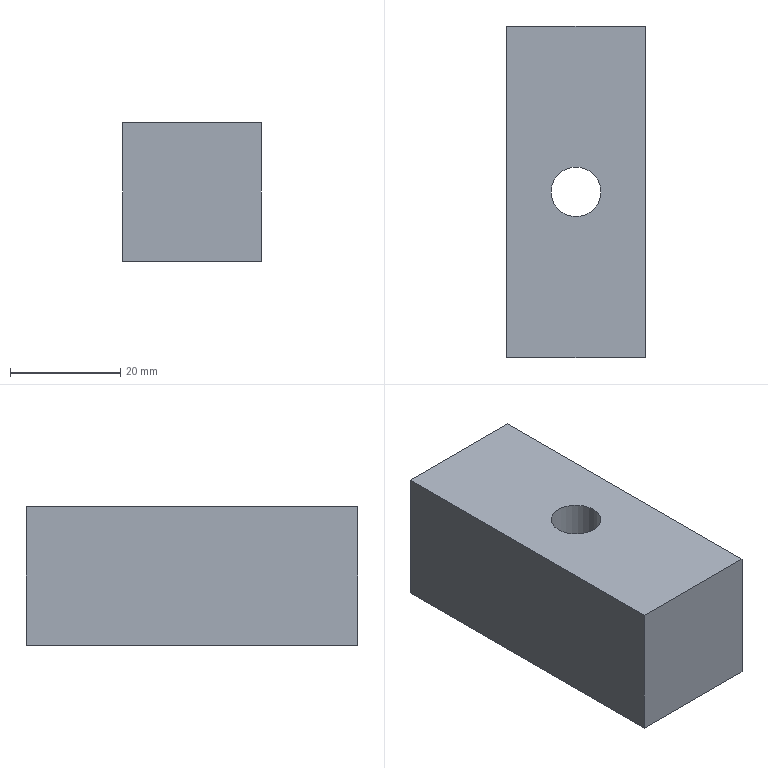Part | NX | features solid 2 | 1 solid | 9 faces | box 25 x 60 x 25 mm | volume 34555 mm3 | plane 7 | cylinder 2 | commonest cylinder face diameters 9 x1 14 x1
STEP:
#1=CARTESIAN_POINT('',(347.,484.5,118.));
#2=VERTEX_POINT('',#1);
#3=CARTESIAN_POINT('',(340.,484.5,118.));
#4=DIRECTION('',(0.,0.,1.));
#5=DIRECTION('',(1.,0.,0.));
#6=AXIS2_PLACEMENT_3D('',#3,#4,#5);
#7=CIRCLE('',#6,7.);
#8=EDGE_CURVE('',#2,#2,#7,.F.);
#9=ORIENTED_EDGE('',*,*,#8,.F.);
#10=EDGE_LOOP('',(#9));
#11=FACE_BOUND('',#10,.T.);
#12=CARTESIAN_POINT('',(327.5,514.5,118.));
#13=VERTEX_POINT('',#12);
#14=CARTESIAN_POINT('',(352.5,514.5,118.));
#15=VERTEX_POINT('',#14);
#16=CARTESIAN_POINT('',(330.,514.5,118.));
#17=DIRECTION('',(-1.,0.,0.));
#18=VECTOR('',#17,1000.);
#19=LINE('',#16,#18);
#20=EDGE_CURVE('',#13,#15,#19,.F.);
#21=ORIENTED_EDGE('',*,*,#20,.T.);
#22=CARTESIAN_POINT('',(352.5,454.5,118.));
#23=VERTEX_POINT('',#22);
#24=CARTESIAN_POINT('',(352.5,510.445,118.));
#25=DIRECTION('',(0.,-1.,0.));
#26=VECTOR('',#25,1000.);
#27=LINE('',#24,#26);
#28=EDGE_CURVE('',#15,#23,#27,.T.);
#29=ORIENTED_EDGE('',*,*,#28,.T.);
#30=CARTESIAN_POINT('',(327.5,454.5,118.));
#31=VERTEX_POINT('',#30);
#32=CARTESIAN_POINT('',(330.,454.5,118.));
#33=DIRECTION('',(1.,0.,0.));
#34=VECTOR('',#33,1000.);
#35=LINE('',#32,#34);
#36=EDGE_CURVE('',#31,#23,#35,.T.);
#37=ORIENTED_EDGE('',*,*,#36,.F.);
#38=CARTESIAN_POINT('',(327.5,510.445,118.));
#39=DIRECTION('',(0.,-1.,0.));
#40=VECTOR('',#39,1000.);
#41=LINE('',#38,#40);
#42=EDGE_CURVE('',#13,#31,#41,.T.);
#43=ORIENTED_EDGE('',*,*,#42,.F.);
#44=EDGE_LOOP('',(#21,#29,#37,#43));
#45=FACE_BOUND('',#44,.T.);
#46=CARTESIAN_POINT('',(330.,510.445,118.));
#47=DIRECTION('',(0.,0.,-1.));
#48=DIRECTION('',(0.,-1.,0.));
#49=AXIS2_PLACEMENT_3D('',#46,#47,#48);
#50=PLANE('',#49);
#51=ADVANCED_FACE('',(#11,#45),#50,.T.);
#52=ORIENTED_EDGE('',*,*,#36,.T.);
#53=CARTESIAN_POINT('',(352.5,454.5,143.));
#54=VERTEX_POINT('',#53);
#55=CARTESIAN_POINT('',(352.5,454.5,123.));
#56=DIRECTION('',(0.,0.,1.));
#57=VECTOR('',#56,1000.);
#58=LINE('',#55,#57);
#59=EDGE_CURVE('',#23,#54,#58,.T.);
#60=ORIENTED_EDGE('',*,*,#59,.T.);
#61=CARTESIAN_POINT('',(327.5,454.5,143.));
#62=VERTEX_POINT('',#61);
#63=CARTESIAN_POINT('',(330.,454.5,143.));
#64=DIRECTION('',(-1.,0.,0.));
#65=VECTOR('',#64,1000.);
#66=LINE('',#63,#65);
#67=EDGE_CURVE('',#62,#54,#66,.F.);
#68=ORIENTED_EDGE('',*,*,#67,.F.);
#69=CARTESIAN_POINT('',(327.5,454.5,123.));
#70=DIRECTION('',(0.,0.,1.));
#71=VECTOR('',#70,1000.);
#72=LINE('',#69,#71);
#73=EDGE_CURVE('',#31,#62,#72,.T.);
#74=ORIENTED_EDGE('',*,*,#73,.F.);
#75=EDGE_LOOP('',(#52,#60,#68,#74));
#76=FACE_BOUND('',#75,.T.);
#77=CARTESIAN_POINT('',(330.,454.5,123.));
#78=DIRECTION('',(0.,-1.,0.));
#79=DIRECTION('',(0.,0.,1.));
#80=AXIS2_PLACEMENT_3D('',#77,#78,#79);
#81=PLANE('',#80);
#82=ADVANCED_FACE('',(#76),#81,.T.);
#83=CARTESIAN_POINT('',(344.5,484.5,143.));
#84=VERTEX_POINT('',#83);
#85=CARTESIAN_POINT('',(340.,484.5,143.));
#86=DIRECTION('',(0.,0.,1.));
#87=DIRECTION('',(1.,0.,0.));
#88=AXIS2_PLACEMENT_3D('',#85,#86,#87);
#89=CIRCLE('',#88,4.5);
#90=EDGE_CURVE('',#84,#84,#89,.F.);
#91=ORIENTED_EDGE('',*,*,#90,.T.);
#92=EDGE_LOOP('',(#91));
#93=FACE_BOUND('',#92,.T.);
#94=ORIENTED_EDGE('',*,*,#67,.T.);
#95=CARTESIAN_POINT('',(352.5,514.5,143.));
#96=VERTEX_POINT('',#95);
#97=CARTESIAN_POINT('',(352.5,510.445,143.));
#98=DIRECTION('',(0.,1.,0.));
#99=VECTOR('',#98,1000.);
#100=LINE('',#97,#99);
#101=EDGE_CURVE('',#96,#54,#100,.F.);
#102=ORIENTED_EDGE('',*,*,#101,.F.);
#103=CARTESIAN_POINT('',(327.5,514.5,143.));
#104=VERTEX_POINT('',#103);
#105=CARTESIAN_POINT('',(330.,514.5,143.));
#106=DIRECTION('',(1.,0.,0.));
#107=VECTOR('',#106,1000.);
#108=LINE('',#105,#107);
#109=EDGE_CURVE('',#104,#96,#108,.T.);
#110=ORIENTED_EDGE('',*,*,#109,.F.);
#111=CARTESIAN_POINT('',(327.5,510.445,143.));
#112=DIRECTION('',(0.,1.,0.));
#113=VECTOR('',#112,1000.);
#114=LINE('',#111,#113);
#115=EDGE_CURVE('',#104,#62,#114,.F.);
#116=ORIENTED_EDGE('',*,*,#115,.T.);
#117=EDGE_LOOP('',(#94,#102,#110,#116));
#118=FACE_BOUND('',#117,.T.);
#119=CARTESIAN_POINT('',(330.,510.445,143.));
#120=DIRECTION('',(0.,0.,-1.));
#121=DIRECTION('',(0.,-1.,0.));
#122=AXIS2_PLACEMENT_3D('',#119,#120,#121);
#123=PLANE('',#122);
#124=ADVANCED_FACE('',(#93,#118),#123,.F.);
#125=CARTESIAN_POINT('',(327.5,514.5,123.));
#126=DIRECTION('',(0.,0.,-1.));
#127=VECTOR('',#126,1000.);
#128=LINE('',#125,#127);
#129=EDGE_CURVE('',#13,#104,#128,.F.);
#130=ORIENTED_EDGE('',*,*,#129,.T.);
#131=ORIENTED_EDGE('',*,*,#109,.T.);
#132=CARTESIAN_POINT('',(352.5,514.5,123.));
#133=DIRECTION('',(0.,0.,-1.));
#134=VECTOR('',#133,1000.);
#135=LINE('',#132,#134);
#136=EDGE_CURVE('',#15,#96,#135,.F.);
#137=ORIENTED_EDGE('',*,*,#136,.F.);
#138=ORIENTED_EDGE('',*,*,#20,.F.);
#139=EDGE_LOOP('',(#130,#131,#137,#138));
#140=FACE_BOUND('',#139,.T.);
#141=CARTESIAN_POINT('',(330.,514.5,123.));
#142=DIRECTION('',(0.,-1.,0.));
#143=DIRECTION('',(0.,0.,1.));
#144=AXIS2_PLACEMENT_3D('',#141,#142,#143);
#145=PLANE('',#144);
#146=ADVANCED_FACE('',(#140),#145,.F.);
#147=ORIENTED_EDGE('',*,*,#101,.T.);
#148=ORIENTED_EDGE('',*,*,#59,.F.);
#149=ORIENTED_EDGE('',*,*,#28,.F.);
#150=ORIENTED_EDGE('',*,*,#136,.T.);
#151=EDGE_LOOP('',(#147,#148,#149,#150));
#152=FACE_BOUND('',#151,.T.);
#153=CARTESIAN_POINT('',(352.5,510.445,123.));
#154=DIRECTION('',(1.,0.,0.));
#155=DIRECTION('',(0.,0.,1.));
#156=AXIS2_PLACEMENT_3D('',#153,#154,#155);
#157=PLANE('',#156);
#158=ADVANCED_FACE('',(#152),#157,.T.);
#159=ORIENTED_EDGE('',*,*,#115,.F.);
#160=ORIENTED_EDGE('',*,*,#129,.F.);
#161=ORIENTED_EDGE('',*,*,#42,.T.);
#162=ORIENTED_EDGE('',*,*,#73,.T.);
#163=EDGE_LOOP('',(#159,#160,#161,#162));
#164=FACE_BOUND('',#163,.T.);
#165=CARTESIAN_POINT('',(327.5,510.445,123.));
#166=DIRECTION('',(1.,0.,0.));
#167=DIRECTION('',(0.,0.,1.));
#168=AXIS2_PLACEMENT_3D('',#165,#166,#167);
#169=PLANE('',#168);
#170=ADVANCED_FACE('',(#164),#169,.F.);
#171=ORIENTED_EDGE('',*,*,#90,.F.);
#172=EDGE_LOOP('',(#171));
#173=FACE_BOUND('',#172,.T.);
#174=CARTESIAN_POINT('',(335.5,484.5,133.));
#175=VERTEX_POINT('',#174);
#176=CARTESIAN_POINT('',(340.,484.5,133.));
#177=DIRECTION('',(0.,0.,-1.));
#178=DIRECTION('',(-1.,0.,0.));
#179=AXIS2_PLACEMENT_3D('',#176,#177,#178);
#180=CIRCLE('',#179,4.5);
#181=EDGE_CURVE('',#175,#175,#180,.T.);
#182=ORIENTED_EDGE('',*,*,#181,.T.);
#183=EDGE_LOOP('',(#182));
#184=FACE_BOUND('',#183,.T.);
#185=CARTESIAN_POINT('',(340.,484.5,173.));
#186=DIRECTION('',(0.,0.,1.));
#187=DIRECTION('',(-1.,0.,0.));
#188=AXIS2_PLACEMENT_3D('',#185,#186,#187);
#189=CYLINDRICAL_SURFACE('',#188,4.5);
#190=ADVANCED_FACE('',(#173,#184),#189,.F.);
#191=ORIENTED_EDGE('',*,*,#181,.F.);
#192=EDGE_LOOP('',(#191));
#193=FACE_BOUND('',#192,.T.);
#194=CARTESIAN_POINT('',(333.,484.5,133.));
#195=VERTEX_POINT('',#194);
#196=CARTESIAN_POINT('',(340.,484.5,133.));
#197=DIRECTION('',(0.,0.,-1.));
#198=DIRECTION('',(-1.,0.,0.));
#199=AXIS2_PLACEMENT_3D('',#196,#197,#198);
#200=CIRCLE('',#199,7.);
#201=EDGE_CURVE('',#195,#195,#200,.T.);
#202=ORIENTED_EDGE('',*,*,#201,.T.);
#203=EDGE_LOOP('',(#202));
#204=FACE_BOUND('',#203,.T.);
#205=CARTESIAN_POINT('',(340.,487.,133.));
#206=DIRECTION('',(0.,0.,1.));
#207=DIRECTION('',(-1.,0.,0.));
#208=AXIS2_PLACEMENT_3D('',#205,#206,#207);
#209=PLANE('',#208);
#210=ADVANCED_FACE('',(#193,#204),#209,.F.);
#211=ORIENTED_EDGE('',*,*,#201,.F.);
#212=EDGE_LOOP('',(#211));
#213=FACE_BOUND('',#212,.T.);
#214=ORIENTED_EDGE('',*,*,#8,.T.);
#215=EDGE_LOOP('',(#214));
#216=FACE_BOUND('',#215,.T.);
#217=CARTESIAN_POINT('',(340.,484.5,123.));
#218=DIRECTION('',(0.,0.,1.));
#219=DIRECTION('',(-1.,0.,0.));
#220=AXIS2_PLACEMENT_3D('',#217,#218,#219);
#221=CYLINDRICAL_SURFACE('',#220,7.);
#222=ADVANCED_FACE('',(#213,#216),#221,.F.);
#223=CLOSED_SHELL('',(#51,#82,#124,#146,#158,#170,#190,#210,#222));
#224=MANIFOLD_SOLID_BREP('',#223);
#225=(LENGTH_UNIT()NAMED_UNIT(*)SI_UNIT(.MILLI.,.METRE.));
#226=UNCERTAINTY_MEASURE_WITH_UNIT(LENGTH_MEASURE(0.00001),#225,'','');
#227=(NAMED_UNIT(*)PLANE_ANGLE_UNIT()SI_UNIT($,.RADIAN.));
#228=(NAMED_UNIT(*)SI_UNIT($,.STERADIAN.)SOLID_ANGLE_UNIT());
#229=(GEOMETRIC_REPRESENTATION_CONTEXT(3)GLOBAL_UNCERTAINTY_ASSIGNED_CONTEXT((#226))GLOBAL_UNIT_ASSIGNED_CONTEXT((#225,#227,#228))REPRESENTATION_CONTEXT('',''));
#230=ADVANCED_BREP_SHAPE_REPRESENTATION('',(#224),#229);